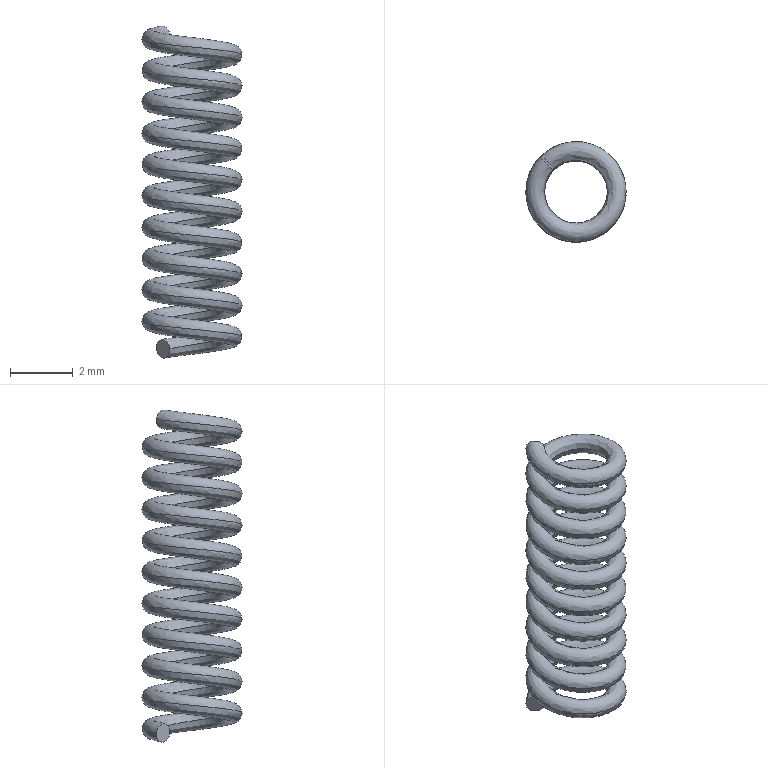Part | SolidWorks | features Helix 1, Sweep 1 | 1 solid | 4 faces | box 3.2 x 3.2 x 10.596 mm | volume 23.105 mm3 | spline 2 | plane 2